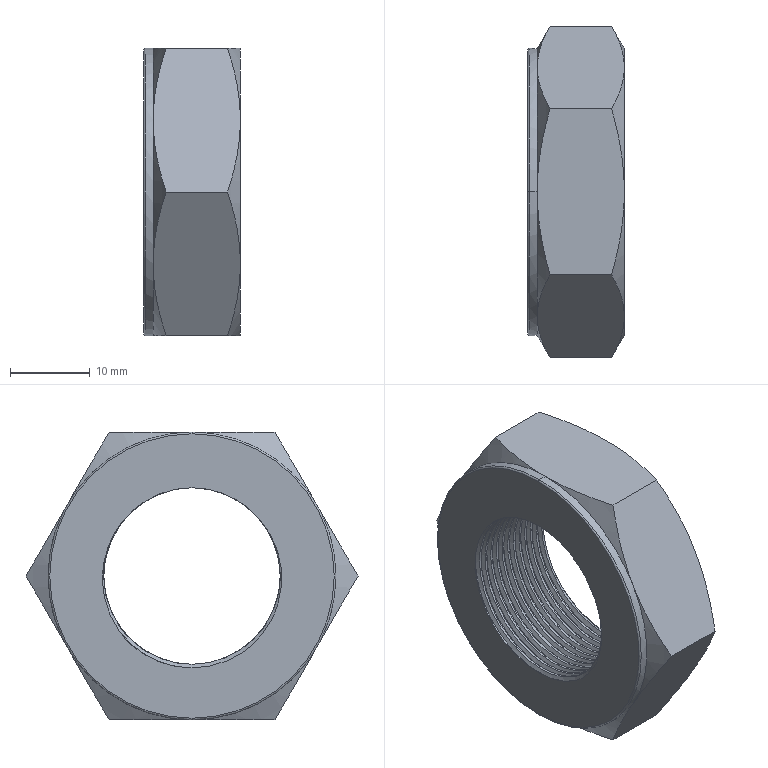Part | STEP file | Completa.sldasm-Part-115_Valor predeterminado | 1 solid | 78 faces | box 12.1 x 41.569 x 36 mm | volume 8539 mm3 | cylinder 54 | cone 12 | plane 8 | torus 2 | spline 2 | commonest cylinder face diameters 22.1 x26 23 x26 36 x2